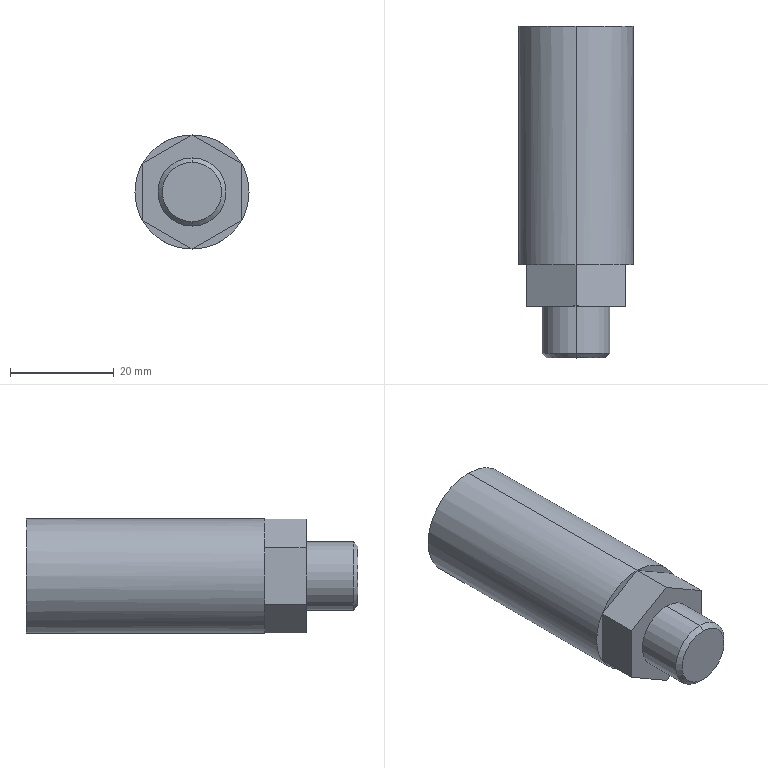Part | SolidWorks | features BaseBody 1 | 1 solid | 16 faces | box 22 x 64 x 22 mm | volume 21333 mm3 | plane 10 | cylinder 4 | cone 2 | commonest cylinder face diameters 13.16 x2 22 x2
STEP:
#1=CARTESIAN_POINT('',(0.,18.,11.));
#2=VERTEX_POINT('',#1);
#3=CARTESIAN_POINT('',(0.,18.,-11.));
#4=VERTEX_POINT('',#3);
#5=CARTESIAN_POINT('',(0.,18.,0.));
#6=DIRECTION('',(0.,1.,0.));
#7=DIRECTION('',(0.,0.,1.));
#8=AXIS2_PLACEMENT_3D('',#5,#6,#7);
#9=CIRCLE('',#8,11.);
#10=EDGE_CURVE('',#2,#4,#9,.T.);
#11=ORIENTED_EDGE('',*,*,#10,.T.);
#12=CARTESIAN_POINT('',(0.,64.,-11.));
#13=VERTEX_POINT('',#12);
#14=CARTESIAN_POINT('',(0.,41.,-11.));
#15=DIRECTION('',(0.,1.,0.));
#16=VECTOR('',#15,1000.);
#17=LINE('',#14,#16);
#18=EDGE_CURVE('',#4,#13,#17,.T.);
#19=ORIENTED_EDGE('',*,*,#18,.T.);
#20=CARTESIAN_POINT('',(0.,64.,11.));
#21=VERTEX_POINT('',#20);
#22=CARTESIAN_POINT('',(0.,64.,0.));
#23=DIRECTION('',(0.,-1.,0.));
#24=DIRECTION('',(0.,0.,1.));
#25=AXIS2_PLACEMENT_3D('',#22,#23,#24);
#26=CIRCLE('',#25,11.);
#27=EDGE_CURVE('',#13,#21,#26,.T.);
#28=ORIENTED_EDGE('',*,*,#27,.T.);
#29=CARTESIAN_POINT('',(0.,41.,11.));
#30=DIRECTION('',(0.,1.,0.));
#31=VECTOR('',#30,1000.);
#32=LINE('',#29,#31);
#33=EDGE_CURVE('',#2,#21,#32,.T.);
#34=ORIENTED_EDGE('',*,*,#33,.F.);
#35=EDGE_LOOP('',(#11,#19,#28,#34));
#36=FACE_OUTER_BOUND('',#35,.T.);
#37=CARTESIAN_POINT('',(0.,41.,0.));
#38=DIRECTION('',(0.,1.,0.));
#39=DIRECTION('',(0.,0.,1.));
#40=AXIS2_PLACEMENT_3D('',#37,#38,#39);
#41=CYLINDRICAL_SURFACE('',#40,11.);
#42=ADVANCED_FACE('',(#36),#41,.T.);
#43=CARTESIAN_POINT('',(0.,0.855,6.58));
#44=VERTEX_POINT('',#43);
#45=CARTESIAN_POINT('',(0.,0.855,-6.58));
#46=VERTEX_POINT('',#45);
#47=CARTESIAN_POINT('',(0.,0.855,0.));
#48=DIRECTION('',(0.,1.,0.));
#49=DIRECTION('',(0.,0.,1.));
#50=AXIS2_PLACEMENT_3D('',#47,#48,#49);
#51=CIRCLE('',#50,6.58);
#52=EDGE_CURVE('',#44,#46,#51,.T.);
#53=ORIENTED_EDGE('',*,*,#52,.T.);
#54=CARTESIAN_POINT('',(0.,10.,-6.58));
#55=VERTEX_POINT('',#54);
#56=CARTESIAN_POINT('',(0.,5.428,-6.58));
#57=DIRECTION('',(0.,1.,0.));
#58=VECTOR('',#57,1000.);
#59=LINE('',#56,#58);
#60=EDGE_CURVE('',#46,#55,#59,.T.);
#61=ORIENTED_EDGE('',*,*,#60,.T.);
#62=CARTESIAN_POINT('',(0.,10.,6.58));
#63=VERTEX_POINT('',#62);
#64=CARTESIAN_POINT('',(0.,10.,0.));
#65=DIRECTION('',(0.,-1.,0.));
#66=DIRECTION('',(0.,0.,1.));
#67=AXIS2_PLACEMENT_3D('',#64,#65,#66);
#68=CIRCLE('',#67,6.58);
#69=EDGE_CURVE('',#55,#63,#68,.T.);
#70=ORIENTED_EDGE('',*,*,#69,.T.);
#71=CARTESIAN_POINT('',(0.,5.428,6.58));
#72=DIRECTION('',(0.,1.,0.));
#73=VECTOR('',#72,1000.);
#74=LINE('',#71,#73);
#75=EDGE_CURVE('',#44,#63,#74,.T.);
#76=ORIENTED_EDGE('',*,*,#75,.F.);
#77=EDGE_LOOP('',(#53,#61,#70,#76));
#78=FACE_OUTER_BOUND('',#77,.T.);
#79=CARTESIAN_POINT('',(0.,5.428,0.));
#80=DIRECTION('',(0.,1.,0.));
#81=DIRECTION('',(0.,0.,1.));
#82=AXIS2_PLACEMENT_3D('',#79,#80,#81);
#83=CYLINDRICAL_SURFACE('',#82,6.58);
#84=ADVANCED_FACE('',(#78),#83,.T.);
#85=CARTESIAN_POINT('',(0.,0.,5.725));
#86=VERTEX_POINT('',#85);
#87=CARTESIAN_POINT('',(0.,0.,-5.725));
#88=VERTEX_POINT('',#87);
#89=CARTESIAN_POINT('',(0.,0.,0.));
#90=DIRECTION('',(0.,1.,0.));
#91=DIRECTION('',(0.,0.,1.));
#92=AXIS2_PLACEMENT_3D('',#89,#90,#91);
#93=CIRCLE('',#92,5.725);
#94=EDGE_CURVE('',#86,#88,#93,.T.);
#95=ORIENTED_EDGE('',*,*,#94,.T.);
#96=CARTESIAN_POINT('',(0.,0.855,-6.58));
#97=DIRECTION('',(0.,0.7071,-0.7071));
#98=VECTOR('',#97,1000.);
#99=LINE('',#96,#98);
#100=EDGE_CURVE('',#88,#46,#99,.T.);
#101=ORIENTED_EDGE('',*,*,#100,.T.);
#102=ORIENTED_EDGE('',*,*,#52,.F.);
#103=CARTESIAN_POINT('',(0.,0.855,6.58));
#104=DIRECTION('',(0.,0.7071,0.7071));
#105=VECTOR('',#104,1000.);
#106=LINE('',#103,#105);
#107=EDGE_CURVE('',#86,#44,#106,.T.);
#108=ORIENTED_EDGE('',*,*,#107,.F.);
#109=EDGE_LOOP('',(#95,#101,#102,#108));
#110=FACE_OUTER_BOUND('',#109,.T.);
#111=CARTESIAN_POINT('',(0.,0.855,0.));
#112=DIRECTION('',(0.,1.,0.));
#113=DIRECTION('',(0.,0.,1.));
#114=AXIS2_PLACEMENT_3D('',#111,#112,#113);
#115=CONICAL_SURFACE('',#114,6.58,0.7854);
#116=ADVANCED_FACE('',(#110),#115,.T.);
#117=ORIENTED_EDGE('',*,*,#18,.F.);
#118=CARTESIAN_POINT('',(0.,18.,0.));
#119=DIRECTION('',(0.,1.,0.));
#120=DIRECTION('',(0.,0.,1.));
#121=AXIS2_PLACEMENT_3D('',#118,#119,#120);
#122=CIRCLE('',#121,11.);
#123=EDGE_CURVE('',#4,#2,#122,.T.);
#124=ORIENTED_EDGE('',*,*,#123,.T.);
#125=ORIENTED_EDGE('',*,*,#33,.T.);
#126=CARTESIAN_POINT('',(0.,64.,0.));
#127=DIRECTION('',(0.,-1.,0.));
#128=DIRECTION('',(0.,0.,1.));
#129=AXIS2_PLACEMENT_3D('',#126,#127,#128);
#130=CIRCLE('',#129,11.);
#131=EDGE_CURVE('',#21,#13,#130,.T.);
#132=ORIENTED_EDGE('',*,*,#131,.T.);
#133=EDGE_LOOP('',(#117,#124,#125,#132));
#134=FACE_OUTER_BOUND('',#133,.T.);
#135=CARTESIAN_POINT('',(0.,41.,0.));
#136=DIRECTION('',(0.,1.,0.));
#137=DIRECTION('',(0.,0.,1.));
#138=AXIS2_PLACEMENT_3D('',#135,#136,#137);
#139=CYLINDRICAL_SURFACE('',#138,11.);
#140=ADVANCED_FACE('',(#134),#139,.T.);
#141=CARTESIAN_POINT('',(-9.5,18.,-5.485));
#142=VERTEX_POINT('',#141);
#143=CARTESIAN_POINT('',(-9.5,18.,5.485));
#144=VERTEX_POINT('',#143);
#145=CARTESIAN_POINT('',(-9.5,18.,0.));
#146=DIRECTION('',(0.,0.,1.));
#147=VECTOR('',#146,1000.);
#148=LINE('',#145,#147);
#149=EDGE_CURVE('',#142,#144,#148,.T.);
#150=ORIENTED_EDGE('',*,*,#149,.T.);
#151=CARTESIAN_POINT('',(0.,18.,10.97));
#152=VERTEX_POINT('',#151);
#153=CARTESIAN_POINT('',(-9.5,18.,5.485));
#154=DIRECTION('',(0.866,0.,0.5));
#155=VECTOR('',#154,1000.);
#156=LINE('',#153,#155);
#157=EDGE_CURVE('',#144,#152,#156,.T.);
#158=ORIENTED_EDGE('',*,*,#157,.T.);
#159=CARTESIAN_POINT('',(9.5,18.,5.485));
#160=VERTEX_POINT('',#159);
#161=CARTESIAN_POINT('',(0.,18.,10.97));
#162=DIRECTION('',(0.866,0.,-0.5));
#163=VECTOR('',#162,1000.);
#164=LINE('',#161,#163);
#165=EDGE_CURVE('',#152,#160,#164,.T.);
#166=ORIENTED_EDGE('',*,*,#165,.T.);
#167=CARTESIAN_POINT('',(9.5,18.,-5.485));
#168=VERTEX_POINT('',#167);
#169=CARTESIAN_POINT('',(9.5,18.,0.));
#170=DIRECTION('',(0.,0.,-1.));
#171=VECTOR('',#170,1000.);
#172=LINE('',#169,#171);
#173=EDGE_CURVE('',#160,#168,#172,.T.);
#174=ORIENTED_EDGE('',*,*,#173,.T.);
#175=CARTESIAN_POINT('',(0.,18.,-10.97));
#176=VERTEX_POINT('',#175);
#177=CARTESIAN_POINT('',(9.5,18.,-5.485));
#178=DIRECTION('',(-0.866,0.,-0.5));
#179=VECTOR('',#178,1000.);
#180=LINE('',#177,#179);
#181=EDGE_CURVE('',#168,#176,#180,.T.);
#182=ORIENTED_EDGE('',*,*,#181,.T.);
#183=CARTESIAN_POINT('',(0.,18.,-10.97));
#184=DIRECTION('',(-0.866,0.,0.5));
#185=VECTOR('',#184,1000.);
#186=LINE('',#183,#185);
#187=EDGE_CURVE('',#176,#142,#186,.T.);
#188=ORIENTED_EDGE('',*,*,#187,.T.);
#189=EDGE_LOOP('',(#150,#158,#166,#174,#182,#188));
#190=FACE_BOUND('',#189,.T.);
#191=ORIENTED_EDGE('',*,*,#10,.F.);
#192=ORIENTED_EDGE('',*,*,#123,.F.);
#193=EDGE_LOOP('',(#191,#192));
#194=FACE_OUTER_BOUND('',#193,.T.);
#195=CARTESIAN_POINT('',(-5.5,18.,0.));
#196=DIRECTION('',(0.,-1.,0.));
#197=DIRECTION('',(0.,0.,-1.));
#198=AXIS2_PLACEMENT_3D('',#195,#196,#197);
#199=PLANE('',#198);
#200=ADVANCED_FACE('',(#190,#194),#199,.T.);
#201=ORIENTED_EDGE('',*,*,#131,.F.);
#202=ORIENTED_EDGE('',*,*,#27,.F.);
#203=EDGE_LOOP('',(#201,#202));
#204=FACE_OUTER_BOUND('',#203,.T.);
#205=CARTESIAN_POINT('',(-5.5,64.,0.));
#206=DIRECTION('',(0.,1.,0.));
#207=DIRECTION('',(0.,0.,1.));
#208=AXIS2_PLACEMENT_3D('',#205,#206,#207);
#209=PLANE('',#208);
#210=ADVANCED_FACE('',(#204),#209,.T.);
#211=CARTESIAN_POINT('',(-9.5,10.,5.485));
#212=VERTEX_POINT('',#211);
#213=CARTESIAN_POINT('',(0.,10.,10.97));
#214=VERTEX_POINT('',#213);
#215=CARTESIAN_POINT('',(0.,10.,10.97));
#216=DIRECTION('',(0.866,0.,0.5));
#217=VECTOR('',#216,1000.);
#218=LINE('',#215,#217);
#219=EDGE_CURVE('',#212,#214,#218,.T.);
#220=ORIENTED_EDGE('',*,*,#219,.T.);
#221=CARTESIAN_POINT('',(0.,10.,10.97));
#222=DIRECTION('',(0.,1.,0.));
#223=VECTOR('',#222,1000.);
#224=LINE('',#221,#223);
#225=EDGE_CURVE('',#214,#152,#224,.T.);
#226=ORIENTED_EDGE('',*,*,#225,.T.);
#227=ORIENTED_EDGE('',*,*,#157,.F.);
#228=CARTESIAN_POINT('',(-9.5,10.,5.485));
#229=DIRECTION('',(0.,-1.,0.));
#230=VECTOR('',#229,1000.);
#231=LINE('',#228,#230);
#232=EDGE_CURVE('',#144,#212,#231,.T.);
#233=ORIENTED_EDGE('',*,*,#232,.T.);
#234=EDGE_LOOP('',(#220,#226,#227,#233));
#235=FACE_OUTER_BOUND('',#234,.T.);
#236=CARTESIAN_POINT('',(0.,10.,10.97));
#237=DIRECTION('',(-0.5,0.,0.866));
#238=DIRECTION('',(0.866,0.,0.5));
#239=AXIS2_PLACEMENT_3D('',#236,#237,#238);
#240=PLANE('',#239);
#241=ADVANCED_FACE('',(#235),#240,.T.);
#242=CARTESIAN_POINT('',(-9.5,10.,-5.485));
#243=VERTEX_POINT('',#242);
#244=CARTESIAN_POINT('',(-9.5,10.,5.485));
#245=DIRECTION('',(0.,0.,1.));
#246=VECTOR('',#245,1000.);
#247=LINE('',#244,#246);
#248=EDGE_CURVE('',#243,#212,#247,.T.);
#249=ORIENTED_EDGE('',*,*,#248,.T.);
#250=ORIENTED_EDGE('',*,*,#232,.F.);
#251=ORIENTED_EDGE('',*,*,#149,.F.);
#252=CARTESIAN_POINT('',(-9.5,10.,-5.485));
#253=DIRECTION('',(0.,-1.,0.));
#254=VECTOR('',#253,1000.);
#255=LINE('',#252,#254);
#256=EDGE_CURVE('',#142,#243,#255,.T.);
#257=ORIENTED_EDGE('',*,*,#256,.T.);
#258=EDGE_LOOP('',(#249,#250,#251,#257));
#259=FACE_OUTER_BOUND('',#258,.T.);
#260=CARTESIAN_POINT('',(-9.5,10.,5.485));
#261=DIRECTION('',(-1.,0.,0.));
#262=DIRECTION('',(0.,0.,1.));
#263=AXIS2_PLACEMENT_3D('',#260,#261,#262);
#264=PLANE('',#263);
#265=ADVANCED_FACE('',(#259),#264,.T.);
#266=CARTESIAN_POINT('',(0.,10.,-10.97));
#267=VERTEX_POINT('',#266);
#268=CARTESIAN_POINT('',(-9.5,10.,-5.485));
#269=DIRECTION('',(-0.866,0.,0.5));
#270=VECTOR('',#269,1000.);
#271=LINE('',#268,#270);
#272=EDGE_CURVE('',#267,#243,#271,.T.);
#273=ORIENTED_EDGE('',*,*,#272,.T.);
#274=ORIENTED_EDGE('',*,*,#256,.F.);
#275=ORIENTED_EDGE('',*,*,#187,.F.);
#276=CARTESIAN_POINT('',(0.,10.,-10.97));
#277=DIRECTION('',(0.,-1.,0.));
#278=VECTOR('',#277,1000.);
#279=LINE('',#276,#278);
#280=EDGE_CURVE('',#176,#267,#279,.T.);
#281=ORIENTED_EDGE('',*,*,#280,.T.);
#282=EDGE_LOOP('',(#273,#274,#275,#281));
#283=FACE_OUTER_BOUND('',#282,.T.);
#284=CARTESIAN_POINT('',(-9.5,10.,-5.485));
#285=DIRECTION('',(-0.5,0.,-0.866));
#286=DIRECTION('',(-0.866,0.,0.5));
#287=AXIS2_PLACEMENT_3D('',#284,#285,#286);
#288=PLANE('',#287);
#289=ADVANCED_FACE('',(#283),#288,.T.);
#290=CARTESIAN_POINT('',(9.5,10.,-5.485));
#291=VERTEX_POINT('',#290);
#292=CARTESIAN_POINT('',(0.,10.,-10.97));
#293=DIRECTION('',(-0.866,0.,-0.5));
#294=VECTOR('',#293,1000.);
#295=LINE('',#292,#294);
#296=EDGE_CURVE('',#291,#267,#295,.T.);
#297=ORIENTED_EDGE('',*,*,#296,.T.);
#298=ORIENTED_EDGE('',*,*,#280,.F.);
#299=ORIENTED_EDGE('',*,*,#181,.F.);
#300=CARTESIAN_POINT('',(9.5,10.,-5.485));
#301=DIRECTION('',(0.,-1.,0.));
#302=VECTOR('',#301,1000.);
#303=LINE('',#300,#302);
#304=EDGE_CURVE('',#168,#291,#303,.T.);
#305=ORIENTED_EDGE('',*,*,#304,.T.);
#306=EDGE_LOOP('',(#297,#298,#299,#305));
#307=FACE_OUTER_BOUND('',#306,.T.);
#308=CARTESIAN_POINT('',(0.,10.,-10.97));
#309=DIRECTION('',(0.5,0.,-0.866));
#310=DIRECTION('',(-0.866,0.,-0.5));
#311=AXIS2_PLACEMENT_3D('',#308,#309,#310);
#312=PLANE('',#311);
#313=ADVANCED_FACE('',(#307),#312,.T.);
#314=CARTESIAN_POINT('',(9.5,10.,5.485));
#315=VERTEX_POINT('',#314);
#316=CARTESIAN_POINT('',(9.5,10.,-5.485));
#317=DIRECTION('',(0.,0.,-1.));
#318=VECTOR('',#317,1000.);
#319=LINE('',#316,#318);
#320=EDGE_CURVE('',#315,#291,#319,.T.);
#321=ORIENTED_EDGE('',*,*,#320,.T.);
#322=ORIENTED_EDGE('',*,*,#304,.F.);
#323=ORIENTED_EDGE('',*,*,#173,.F.);
#324=CARTESIAN_POINT('',(9.5,10.,5.485));
#325=DIRECTION('',(0.,-1.,0.));
#326=VECTOR('',#325,1000.);
#327=LINE('',#324,#326);
#328=EDGE_CURVE('',#160,#315,#327,.T.);
#329=ORIENTED_EDGE('',*,*,#328,.T.);
#330=EDGE_LOOP('',(#321,#322,#323,#329));
#331=FACE_OUTER_BOUND('',#330,.T.);
#332=CARTESIAN_POINT('',(9.5,10.,-5.485));
#333=DIRECTION('',(1.,0.,0.));
#334=DIRECTION('',(0.,0.,-1.));
#335=AXIS2_PLACEMENT_3D('',#332,#333,#334);
#336=PLANE('',#335);
#337=ADVANCED_FACE('',(#331),#336,.T.);
#338=CARTESIAN_POINT('',(9.5,10.,5.485));
#339=DIRECTION('',(0.866,0.,-0.5));
#340=VECTOR('',#339,1000.);
#341=LINE('',#338,#340);
#342=EDGE_CURVE('',#214,#315,#341,.T.);
#343=ORIENTED_EDGE('',*,*,#342,.T.);
#344=ORIENTED_EDGE('',*,*,#328,.F.);
#345=ORIENTED_EDGE('',*,*,#165,.F.);
#346=ORIENTED_EDGE('',*,*,#225,.F.);
#347=EDGE_LOOP('',(#343,#344,#345,#346));
#348=FACE_OUTER_BOUND('',#347,.T.);
#349=CARTESIAN_POINT('',(9.5,10.,5.485));
#350=DIRECTION('',(0.5,0.,0.866));
#351=DIRECTION('',(0.866,0.,-0.5));
#352=AXIS2_PLACEMENT_3D('',#349,#350,#351);
#353=PLANE('',#352);
#354=ADVANCED_FACE('',(#348),#353,.T.);
#355=CARTESIAN_POINT('',(0.,10.,0.));
#356=DIRECTION('',(0.,-1.,0.));
#357=DIRECTION('',(0.,0.,1.));
#358=AXIS2_PLACEMENT_3D('',#355,#356,#357);
#359=CIRCLE('',#358,6.58);
#360=EDGE_CURVE('',#63,#55,#359,.T.);
#361=ORIENTED_EDGE('',*,*,#360,.F.);
#362=ORIENTED_EDGE('',*,*,#69,.F.);
#363=EDGE_LOOP('',(#361,#362));
#364=FACE_BOUND('',#363,.T.);
#365=ORIENTED_EDGE('',*,*,#342,.F.);
#366=ORIENTED_EDGE('',*,*,#219,.F.);
#367=ORIENTED_EDGE('',*,*,#248,.F.);
#368=ORIENTED_EDGE('',*,*,#272,.F.);
#369=ORIENTED_EDGE('',*,*,#296,.F.);
#370=ORIENTED_EDGE('',*,*,#320,.F.);
#371=EDGE_LOOP('',(#365,#366,#367,#368,#369,#370));
#372=FACE_OUTER_BOUND('',#371,.T.);
#373=CARTESIAN_POINT('',(0.,10.,0.));
#374=DIRECTION('',(0.,1.,0.));
#375=DIRECTION('',(0.,0.,1.));
#376=AXIS2_PLACEMENT_3D('',#373,#374,#375);
#377=PLANE('',#376);
#378=ADVANCED_FACE('',(#364,#372),#377,.F.);
#379=ORIENTED_EDGE('',*,*,#60,.F.);
#380=CARTESIAN_POINT('',(0.,0.855,0.));
#381=DIRECTION('',(0.,1.,0.));
#382=DIRECTION('',(0.,0.,1.));
#383=AXIS2_PLACEMENT_3D('',#380,#381,#382);
#384=CIRCLE('',#383,6.58);
#385=EDGE_CURVE('',#46,#44,#384,.T.);
#386=ORIENTED_EDGE('',*,*,#385,.T.);
#387=ORIENTED_EDGE('',*,*,#75,.T.);
#388=ORIENTED_EDGE('',*,*,#360,.T.);
#389=EDGE_LOOP('',(#379,#386,#387,#388));
#390=FACE_OUTER_BOUND('',#389,.T.);
#391=CARTESIAN_POINT('',(0.,5.428,0.));
#392=DIRECTION('',(0.,1.,0.));
#393=DIRECTION('',(0.,0.,1.));
#394=AXIS2_PLACEMENT_3D('',#391,#392,#393);
#395=CYLINDRICAL_SURFACE('',#394,6.58);
#396=ADVANCED_FACE('',(#390),#395,.T.);
#397=ORIENTED_EDGE('',*,*,#100,.F.);
#398=CARTESIAN_POINT('',(0.,0.,0.));
#399=DIRECTION('',(0.,1.,0.));
#400=DIRECTION('',(0.,0.,1.));
#401=AXIS2_PLACEMENT_3D('',#398,#399,#400);
#402=CIRCLE('',#401,5.725);
#403=EDGE_CURVE('',#88,#86,#402,.T.);
#404=ORIENTED_EDGE('',*,*,#403,.T.);
#405=ORIENTED_EDGE('',*,*,#107,.T.);
#406=ORIENTED_EDGE('',*,*,#385,.F.);
#407=EDGE_LOOP('',(#397,#404,#405,#406));
#408=FACE_OUTER_BOUND('',#407,.T.);
#409=CARTESIAN_POINT('',(0.,0.855,0.));
#410=DIRECTION('',(0.,1.,0.));
#411=DIRECTION('',(0.,0.,1.));
#412=AXIS2_PLACEMENT_3D('',#409,#410,#411);
#413=CONICAL_SURFACE('',#412,6.58,0.7854);
#414=ADVANCED_FACE('',(#408),#413,.T.);
#415=ORIENTED_EDGE('',*,*,#94,.F.);
#416=ORIENTED_EDGE('',*,*,#403,.F.);
#417=EDGE_LOOP('',(#415,#416));
#418=FACE_OUTER_BOUND('',#417,.T.);
#419=CARTESIAN_POINT('',(-2.862,0.,0.));
#420=DIRECTION('',(0.,-1.,0.));
#421=DIRECTION('',(0.,0.,-1.));
#422=AXIS2_PLACEMENT_3D('',#419,#420,#421);
#423=PLANE('',#422);
#424=ADVANCED_FACE('',(#418),#423,.T.);
#425=CLOSED_SHELL('',(#42,#84,#116,#140,#200,#210,#241,#265,#289,#313,#337,#354,#378,#396,#414,#424));
#426=MANIFOLD_SOLID_BREP('',#425);
#427=CARTESIAN_POINT('',(0.,0.,0.));
#428=DIRECTION('',(0.,0.,1.));
#429=DIRECTION('',(1.,0.,0.));
#430=AXIS2_PLACEMENT_3D('',#427,#428,#429);
#431=(LENGTH_UNIT()NAMED_UNIT(*)SI_UNIT(.MILLI.,.METRE.));
#432=UNCERTAINTY_MEASURE_WITH_UNIT(LENGTH_MEASURE(0.00001),#431,'','');
#433=(NAMED_UNIT(*)PLANE_ANGLE_UNIT()SI_UNIT($,.RADIAN.));
#434=(NAMED_UNIT(*)SI_UNIT($,.STERADIAN.)SOLID_ANGLE_UNIT());
#435=(GEOMETRIC_REPRESENTATION_CONTEXT(3)GLOBAL_UNCERTAINTY_ASSIGNED_CONTEXT((#432))GLOBAL_UNIT_ASSIGNED_CONTEXT((#431,#433,#434))REPRESENTATION_CONTEXT('',''));
#436=ADVANCED_BREP_SHAPE_REPRESENTATION('',(#426,#430),#435);